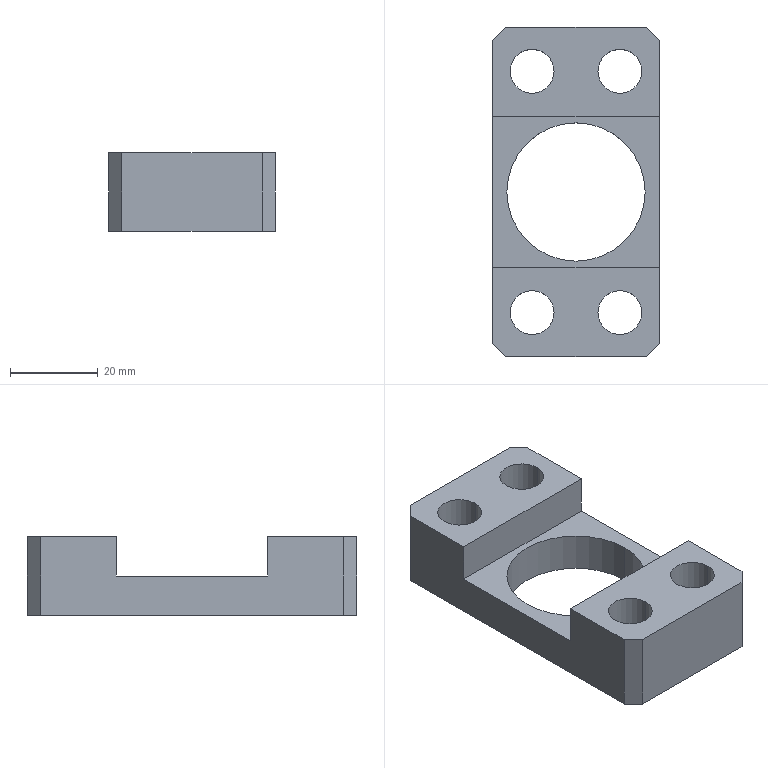Part | STEP file | Floating joint mounting plate | 1 solid | 36 faces | box 38 x 75 x 18 mm | volume 24096 mm3 | plane 18 | cylinder 18 | commonest cylinder face diameters 10 x8 14 x8 31.5 x2
STEP:
#1=CARTESIAN_POINT('',(34.75,37.5,9.));
#2=VERTEX_POINT('',#1);
#3=CARTESIAN_POINT('',(3.25,37.5,9.));
#4=VERTEX_POINT('',#3);
#5=CARTESIAN_POINT('',(19.,37.5,9.));
#6=DIRECTION('',(0.,0.,1.));
#7=DIRECTION('',(1.,0.,0.));
#8=AXIS2_PLACEMENT_3D('',#5,#6,#7);
#9=CIRCLE('',#8,15.75);
#10=EDGE_CURVE('',#2,#4,#9,.T.);
#11=ORIENTED_EDGE('',*,*,#10,.F.);
#12=CARTESIAN_POINT('',(19.,37.5,9.));
#13=DIRECTION('',(0.,0.,1.));
#14=DIRECTION('',(1.,0.,0.));
#15=AXIS2_PLACEMENT_3D('',#12,#13,#14);
#16=CIRCLE('',#15,15.75);
#17=EDGE_CURVE('',#4,#2,#16,.T.);
#18=ORIENTED_EDGE('',*,*,#17,.F.);
#19=EDGE_LOOP('',(#11,#18));
#20=FACE_BOUND('',#19,.T.);
#21=CARTESIAN_POINT('',(0.,20.25,9.));
#22=VERTEX_POINT('',#21);
#23=CARTESIAN_POINT('',(0.,54.75,9.));
#24=VERTEX_POINT('',#23);
#25=CARTESIAN_POINT('',(0.,20.25,9.));
#26=DIRECTION('',(0.,1.,0.));
#27=VECTOR('',#26,1000.);
#28=LINE('',#25,#27);
#29=EDGE_CURVE('',#22,#24,#28,.T.);
#30=ORIENTED_EDGE('',*,*,#29,.F.);
#31=CARTESIAN_POINT('',(38.,20.25,9.));
#32=VERTEX_POINT('',#31);
#33=CARTESIAN_POINT('',(38.,20.25,9.));
#34=DIRECTION('',(-1.,0.,0.));
#35=VECTOR('',#34,1000.);
#36=LINE('',#33,#35);
#37=EDGE_CURVE('',#32,#22,#36,.T.);
#38=ORIENTED_EDGE('',*,*,#37,.F.);
#39=CARTESIAN_POINT('',(38.,54.75,9.));
#40=VERTEX_POINT('',#39);
#41=CARTESIAN_POINT('',(38.,20.25,9.));
#42=DIRECTION('',(0.,1.,0.));
#43=VECTOR('',#42,1000.);
#44=LINE('',#41,#43);
#45=EDGE_CURVE('',#32,#40,#44,.T.);
#46=ORIENTED_EDGE('',*,*,#45,.T.);
#47=CARTESIAN_POINT('',(38.,54.75,9.));
#48=DIRECTION('',(-1.,0.,0.));
#49=VECTOR('',#48,1000.);
#50=LINE('',#47,#49);
#51=EDGE_CURVE('',#40,#24,#50,.T.);
#52=ORIENTED_EDGE('',*,*,#51,.T.);
#53=EDGE_LOOP('',(#30,#38,#46,#52));
#54=FACE_OUTER_BOUND('',#53,.T.);
#55=CARTESIAN_POINT('',(38.,20.25,9.));
#56=DIRECTION('',(0.,0.,1.));
#57=DIRECTION('',(1.,0.,0.));
#58=AXIS2_PLACEMENT_3D('',#55,#56,#57);
#59=PLANE('',#58);
#60=ADVANCED_FACE('',(#20,#54),#59,.T.);
#61=CARTESIAN_POINT('',(0.,54.75,18.));
#62=VERTEX_POINT('',#61);
#63=CARTESIAN_POINT('',(0.,54.75,9.));
#64=DIRECTION('',(0.,0.,1.));
#65=VECTOR('',#64,1000.);
#66=LINE('',#63,#65);
#67=EDGE_CURVE('',#24,#62,#66,.T.);
#68=ORIENTED_EDGE('',*,*,#67,.F.);
#69=ORIENTED_EDGE('',*,*,#51,.F.);
#70=CARTESIAN_POINT('',(38.,54.75,18.));
#71=VERTEX_POINT('',#70);
#72=CARTESIAN_POINT('',(38.,54.75,9.));
#73=DIRECTION('',(0.,0.,1.));
#74=VECTOR('',#73,1000.);
#75=LINE('',#72,#74);
#76=EDGE_CURVE('',#40,#71,#75,.T.);
#77=ORIENTED_EDGE('',*,*,#76,.T.);
#78=CARTESIAN_POINT('',(0.,54.75,18.));
#79=DIRECTION('',(1.,0.,0.));
#80=VECTOR('',#79,1000.);
#81=LINE('',#78,#80);
#82=EDGE_CURVE('',#62,#71,#81,.T.);
#83=ORIENTED_EDGE('',*,*,#82,.F.);
#84=EDGE_LOOP('',(#68,#69,#77,#83));
#85=FACE_OUTER_BOUND('',#84,.T.);
#86=CARTESIAN_POINT('',(38.,54.75,9.));
#87=DIRECTION('',(0.,-1.,0.));
#88=DIRECTION('',(0.,0.,-1.));
#89=AXIS2_PLACEMENT_3D('',#86,#87,#88);
#90=PLANE('',#89);
#91=ADVANCED_FACE('',(#85),#90,.T.);
#92=CARTESIAN_POINT('',(24.,65.,18.));
#93=VERTEX_POINT('',#92);
#94=CARTESIAN_POINT('',(34.,65.,18.));
#95=VERTEX_POINT('',#94);
#96=CARTESIAN_POINT('',(29.,65.,18.));
#97=DIRECTION('',(0.,0.,-1.));
#98=DIRECTION('',(-1.,0.,0.));
#99=AXIS2_PLACEMENT_3D('',#96,#97,#98);
#100=CIRCLE('',#99,5.);
#101=EDGE_CURVE('',#93,#95,#100,.T.);
#102=ORIENTED_EDGE('',*,*,#101,.T.);
#103=CARTESIAN_POINT('',(29.,65.,18.));
#104=DIRECTION('',(0.,0.,-1.));
#105=DIRECTION('',(-1.,0.,0.));
#106=AXIS2_PLACEMENT_3D('',#103,#104,#105);
#107=CIRCLE('',#106,5.);
#108=EDGE_CURVE('',#95,#93,#107,.T.);
#109=ORIENTED_EDGE('',*,*,#108,.T.);
#110=EDGE_LOOP('',(#102,#109));
#111=FACE_BOUND('',#110,.T.);
#112=CARTESIAN_POINT('',(4.,65.,18.));
#113=VERTEX_POINT('',#112);
#114=CARTESIAN_POINT('',(14.,65.,18.));
#115=VERTEX_POINT('',#114);
#116=CARTESIAN_POINT('',(9.,65.,18.));
#117=DIRECTION('',(0.,0.,-1.));
#118=DIRECTION('',(-1.,0.,0.));
#119=AXIS2_PLACEMENT_3D('',#116,#117,#118);
#120=CIRCLE('',#119,5.);
#121=EDGE_CURVE('',#113,#115,#120,.T.);
#122=ORIENTED_EDGE('',*,*,#121,.T.);
#123=CARTESIAN_POINT('',(9.,65.,18.));
#124=DIRECTION('',(0.,0.,-1.));
#125=DIRECTION('',(-1.,0.,0.));
#126=AXIS2_PLACEMENT_3D('',#123,#124,#125);
#127=CIRCLE('',#126,5.);
#128=EDGE_CURVE('',#115,#113,#127,.T.);
#129=ORIENTED_EDGE('',*,*,#128,.T.);
#130=EDGE_LOOP('',(#122,#129));
#131=FACE_BOUND('',#130,.T.);
#132=CARTESIAN_POINT('',(0.,72.,18.));
#133=VERTEX_POINT('',#132);
#134=CARTESIAN_POINT('',(0.,72.,18.));
#135=DIRECTION('',(0.,-1.,0.));
#136=VECTOR('',#135,1000.);
#137=LINE('',#134,#136);
#138=EDGE_CURVE('',#133,#62,#137,.T.);
#139=ORIENTED_EDGE('',*,*,#138,.T.);
#140=ORIENTED_EDGE('',*,*,#82,.T.);
#141=CARTESIAN_POINT('',(38.,72.,18.));
#142=VERTEX_POINT('',#141);
#143=CARTESIAN_POINT('',(38.,3.,18.));
#144=DIRECTION('',(0.,1.,0.));
#145=VECTOR('',#144,1000.);
#146=LINE('',#143,#145);
#147=EDGE_CURVE('',#71,#142,#146,.T.);
#148=ORIENTED_EDGE('',*,*,#147,.T.);
#149=CARTESIAN_POINT('',(35.,75.,18.));
#150=VERTEX_POINT('',#149);
#151=CARTESIAN_POINT('',(38.,72.,18.));
#152=DIRECTION('',(-0.7071,0.7071,0.));
#153=VECTOR('',#152,1000.);
#154=LINE('',#151,#153);
#155=EDGE_CURVE('',#142,#150,#154,.T.);
#156=ORIENTED_EDGE('',*,*,#155,.T.);
#157=CARTESIAN_POINT('',(3.,75.,18.));
#158=VERTEX_POINT('',#157);
#159=CARTESIAN_POINT('',(35.,75.,18.));
#160=DIRECTION('',(-1.,0.,0.));
#161=VECTOR('',#160,1000.);
#162=LINE('',#159,#161);
#163=EDGE_CURVE('',#150,#158,#162,.T.);
#164=ORIENTED_EDGE('',*,*,#163,.T.);
#165=CARTESIAN_POINT('',(3.,75.,18.));
#166=DIRECTION('',(-0.7071,-0.7071,0.));
#167=VECTOR('',#166,1000.);
#168=LINE('',#165,#167);
#169=EDGE_CURVE('',#158,#133,#168,.T.);
#170=ORIENTED_EDGE('',*,*,#169,.T.);
#171=EDGE_LOOP('',(#139,#140,#148,#156,#164,#170));
#172=FACE_OUTER_BOUND('',#171,.T.);
#173=CARTESIAN_POINT('',(0.,0.,18.));
#174=DIRECTION('',(0.,0.,1.));
#175=DIRECTION('',(1.,0.,0.));
#176=AXIS2_PLACEMENT_3D('',#173,#174,#175);
#177=PLANE('',#176);
#178=ADVANCED_FACE('',(#111,#131,#172),#177,.T.);
#179=CARTESIAN_POINT('',(3.,75.,0.));
#180=VERTEX_POINT('',#179);
#181=CARTESIAN_POINT('',(0.,72.,0.));
#182=VERTEX_POINT('',#181);
#183=CARTESIAN_POINT('',(3.,75.,0.));
#184=DIRECTION('',(-0.7071,-0.7071,0.));
#185=VECTOR('',#184,1000.);
#186=LINE('',#183,#185);
#187=EDGE_CURVE('',#180,#182,#186,.T.);
#188=ORIENTED_EDGE('',*,*,#187,.T.);
#189=CARTESIAN_POINT('',(0.,72.,18.));
#190=DIRECTION('',(0.,0.,-1.));
#191=VECTOR('',#190,1000.);
#192=LINE('',#189,#191);
#193=EDGE_CURVE('',#133,#182,#192,.T.);
#194=ORIENTED_EDGE('',*,*,#193,.F.);
#195=ORIENTED_EDGE('',*,*,#169,.F.);
#196=CARTESIAN_POINT('',(3.,75.,18.));
#197=DIRECTION('',(0.,0.,-1.));
#198=VECTOR('',#197,1000.);
#199=LINE('',#196,#198);
#200=EDGE_CURVE('',#158,#180,#199,.T.);
#201=ORIENTED_EDGE('',*,*,#200,.T.);
#202=EDGE_LOOP('',(#188,#194,#195,#201));
#203=FACE_OUTER_BOUND('',#202,.T.);
#204=CARTESIAN_POINT('',(3.,75.,18.));
#205=DIRECTION('',(0.7071,-0.7071,0.));
#206=DIRECTION('',(0.7071,0.7071,0.));
#207=AXIS2_PLACEMENT_3D('',#204,#205,#206);
#208=PLANE('',#207);
#209=ADVANCED_FACE('',(#203),#208,.F.);
#210=CARTESIAN_POINT('',(35.,75.,0.));
#211=VERTEX_POINT('',#210);
#212=CARTESIAN_POINT('',(35.,75.,0.));
#213=DIRECTION('',(-1.,0.,0.));
#214=VECTOR('',#213,1000.);
#215=LINE('',#212,#214);
#216=EDGE_CURVE('',#211,#180,#215,.T.);
#217=ORIENTED_EDGE('',*,*,#216,.T.);
#218=ORIENTED_EDGE('',*,*,#200,.F.);
#219=ORIENTED_EDGE('',*,*,#163,.F.);
#220=CARTESIAN_POINT('',(35.,75.,18.));
#221=DIRECTION('',(0.,0.,-1.));
#222=VECTOR('',#221,1000.);
#223=LINE('',#220,#222);
#224=EDGE_CURVE('',#150,#211,#223,.T.);
#225=ORIENTED_EDGE('',*,*,#224,.T.);
#226=EDGE_LOOP('',(#217,#218,#219,#225));
#227=FACE_OUTER_BOUND('',#226,.T.);
#228=CARTESIAN_POINT('',(35.,75.,18.));
#229=DIRECTION('',(0.,-1.,0.));
#230=DIRECTION('',(0.,0.,-1.));
#231=AXIS2_PLACEMENT_3D('',#228,#229,#230);
#232=PLANE('',#231);
#233=ADVANCED_FACE('',(#227),#232,.F.);
#234=CARTESIAN_POINT('',(38.,72.,0.));
#235=VERTEX_POINT('',#234);
#236=CARTESIAN_POINT('',(38.,72.,0.));
#237=DIRECTION('',(-0.7071,0.7071,0.));
#238=VECTOR('',#237,1000.);
#239=LINE('',#236,#238);
#240=EDGE_CURVE('',#235,#211,#239,.T.);
#241=ORIENTED_EDGE('',*,*,#240,.T.);
#242=ORIENTED_EDGE('',*,*,#224,.F.);
#243=ORIENTED_EDGE('',*,*,#155,.F.);
#244=CARTESIAN_POINT('',(38.,72.,18.));
#245=DIRECTION('',(0.,0.,-1.));
#246=VECTOR('',#245,1000.);
#247=LINE('',#244,#246);
#248=EDGE_CURVE('',#142,#235,#247,.T.);
#249=ORIENTED_EDGE('',*,*,#248,.T.);
#250=EDGE_LOOP('',(#241,#242,#243,#249));
#251=FACE_OUTER_BOUND('',#250,.T.);
#252=CARTESIAN_POINT('',(38.,72.,18.));
#253=DIRECTION('',(-0.7071,-0.7071,0.));
#254=DIRECTION('',(0.7071,-0.7071,0.));
#255=AXIS2_PLACEMENT_3D('',#252,#253,#254);
#256=PLANE('',#255);
#257=ADVANCED_FACE('',(#251),#256,.F.);
#258=ORIENTED_EDGE('',*,*,#76,.F.);
#259=ORIENTED_EDGE('',*,*,#45,.F.);
#260=CARTESIAN_POINT('',(38.,20.25,18.));
#261=VERTEX_POINT('',#260);
#262=CARTESIAN_POINT('',(38.,20.25,22.5));
#263=DIRECTION('',(0.,0.,-1.));
#264=VECTOR('',#263,1000.);
#265=LINE('',#262,#264);
#266=EDGE_CURVE('',#261,#32,#265,.T.);
#267=ORIENTED_EDGE('',*,*,#266,.F.);
#268=CARTESIAN_POINT('',(38.,3.,18.));
#269=VERTEX_POINT('',#268);
#270=CARTESIAN_POINT('',(38.,3.,18.));
#271=DIRECTION('',(0.,1.,0.));
#272=VECTOR('',#271,1000.);
#273=LINE('',#270,#272);
#274=EDGE_CURVE('',#269,#261,#273,.T.);
#275=ORIENTED_EDGE('',*,*,#274,.F.);
#276=CARTESIAN_POINT('',(38.,3.,0.));
#277=VERTEX_POINT('',#276);
#278=CARTESIAN_POINT('',(38.,3.,18.));
#279=DIRECTION('',(0.,0.,-1.));
#280=VECTOR('',#279,1000.);
#281=LINE('',#278,#280);
#282=EDGE_CURVE('',#269,#277,#281,.T.);
#283=ORIENTED_EDGE('',*,*,#282,.T.);
#284=CARTESIAN_POINT('',(38.,3.,0.));
#285=DIRECTION('',(0.,1.,0.));
#286=VECTOR('',#285,1000.);
#287=LINE('',#284,#286);
#288=EDGE_CURVE('',#277,#235,#287,.T.);
#289=ORIENTED_EDGE('',*,*,#288,.T.);
#290=ORIENTED_EDGE('',*,*,#248,.F.);
#291=ORIENTED_EDGE('',*,*,#147,.F.);
#292=EDGE_LOOP('',(#258,#259,#267,#275,#283,#289,#290,#291));
#293=FACE_OUTER_BOUND('',#292,.T.);
#294=CARTESIAN_POINT('',(38.,3.,18.));
#295=DIRECTION('',(-1.,0.,0.));
#296=DIRECTION('',(0.,0.,1.));
#297=AXIS2_PLACEMENT_3D('',#294,#295,#296);
#298=PLANE('',#297);
#299=ADVANCED_FACE('',(#293),#298,.F.);
#300=CARTESIAN_POINT('',(22.,65.,0.));
#301=VERTEX_POINT('',#300);
#302=CARTESIAN_POINT('',(36.,65.,0.));
#303=VERTEX_POINT('',#302);
#304=CARTESIAN_POINT('',(29.,65.,0.));
#305=DIRECTION('',(0.,0.,-1.));
#306=DIRECTION('',(-1.,0.,0.));
#307=AXIS2_PLACEMENT_3D('',#304,#305,#306);
#308=CIRCLE('',#307,7.);
#309=EDGE_CURVE('',#301,#303,#308,.T.);
#310=ORIENTED_EDGE('',*,*,#309,.F.);
#311=CARTESIAN_POINT('',(29.,65.,0.));
#312=DIRECTION('',(0.,0.,-1.));
#313=DIRECTION('',(-1.,0.,0.));
#314=AXIS2_PLACEMENT_3D('',#311,#312,#313);
#315=CIRCLE('',#314,7.);
#316=EDGE_CURVE('',#303,#301,#315,.T.);
#317=ORIENTED_EDGE('',*,*,#316,.F.);
#318=EDGE_LOOP('',(#310,#317));
#319=FACE_BOUND('',#318,.T.);
#320=CARTESIAN_POINT('',(2.,10.,0.));
#321=VERTEX_POINT('',#320);
#322=CARTESIAN_POINT('',(16.,10.,0.));
#323=VERTEX_POINT('',#322);
#324=CARTESIAN_POINT('',(9.,10.,0.));
#325=DIRECTION('',(0.,0.,-1.));
#326=DIRECTION('',(-1.,0.,0.));
#327=AXIS2_PLACEMENT_3D('',#324,#325,#326);
#328=CIRCLE('',#327,7.);
#329=EDGE_CURVE('',#321,#323,#328,.T.);
#330=ORIENTED_EDGE('',*,*,#329,.F.);
#331=CARTESIAN_POINT('',(9.,10.,0.));
#332=DIRECTION('',(0.,0.,-1.));
#333=DIRECTION('',(-1.,0.,0.));
#334=AXIS2_PLACEMENT_3D('',#331,#332,#333);
#335=CIRCLE('',#334,7.);
#336=EDGE_CURVE('',#323,#321,#335,.T.);
#337=ORIENTED_EDGE('',*,*,#336,.F.);
#338=EDGE_LOOP('',(#330,#337));
#339=FACE_BOUND('',#338,.T.);
#340=CARTESIAN_POINT('',(22.,10.,0.));
#341=VERTEX_POINT('',#340);
#342=CARTESIAN_POINT('',(36.,10.,0.));
#343=VERTEX_POINT('',#342);
#344=CARTESIAN_POINT('',(29.,10.,0.));
#345=DIRECTION('',(0.,0.,-1.));
#346=DIRECTION('',(-1.,0.,0.));
#347=AXIS2_PLACEMENT_3D('',#344,#345,#346);
#348=CIRCLE('',#347,7.);
#349=EDGE_CURVE('',#341,#343,#348,.T.);
#350=ORIENTED_EDGE('',*,*,#349,.F.);
#351=CARTESIAN_POINT('',(29.,10.,0.));
#352=DIRECTION('',(0.,0.,-1.));
#353=DIRECTION('',(-1.,0.,0.));
#354=AXIS2_PLACEMENT_3D('',#351,#352,#353);
#355=CIRCLE('',#354,7.);
#356=EDGE_CURVE('',#343,#341,#355,.T.);
#357=ORIENTED_EDGE('',*,*,#356,.F.);
#358=EDGE_LOOP('',(#350,#357));
#359=FACE_BOUND('',#358,.T.);
#360=CARTESIAN_POINT('',(2.,65.,0.));
#361=VERTEX_POINT('',#360);
#362=CARTESIAN_POINT('',(16.,65.,0.));
#363=VERTEX_POINT('',#362);
#364=CARTESIAN_POINT('',(9.,65.,0.));
#365=DIRECTION('',(0.,0.,-1.));
#366=DIRECTION('',(-1.,0.,0.));
#367=AXIS2_PLACEMENT_3D('',#364,#365,#366);
#368=CIRCLE('',#367,7.);
#369=EDGE_CURVE('',#361,#363,#368,.T.);
#370=ORIENTED_EDGE('',*,*,#369,.F.);
#371=CARTESIAN_POINT('',(9.,65.,0.));
#372=DIRECTION('',(0.,0.,-1.));
#373=DIRECTION('',(-1.,0.,0.));
#374=AXIS2_PLACEMENT_3D('',#371,#372,#373);
#375=CIRCLE('',#374,7.);
#376=EDGE_CURVE('',#363,#361,#375,.T.);
#377=ORIENTED_EDGE('',*,*,#376,.F.);
#378=EDGE_LOOP('',(#370,#377));
#379=FACE_BOUND('',#378,.T.);
#380=CARTESIAN_POINT('',(34.75,37.5,0.));
#381=VERTEX_POINT('',#380);
#382=CARTESIAN_POINT('',(3.25,37.5,0.));
#383=VERTEX_POINT('',#382);
#384=CARTESIAN_POINT('',(19.,37.5,0.));
#385=DIRECTION('',(0.,0.,1.));
#386=DIRECTION('',(1.,0.,0.));
#387=AXIS2_PLACEMENT_3D('',#384,#385,#386);
#388=CIRCLE('',#387,15.75);
#389=EDGE_CURVE('',#381,#383,#388,.T.);
#390=ORIENTED_EDGE('',*,*,#389,.T.);
#391=CARTESIAN_POINT('',(19.,37.5,0.));
#392=DIRECTION('',(0.,0.,1.));
#393=DIRECTION('',(1.,0.,0.));
#394=AXIS2_PLACEMENT_3D('',#391,#392,#393);
#395=CIRCLE('',#394,15.75);
#396=EDGE_CURVE('',#383,#381,#395,.T.);
#397=ORIENTED_EDGE('',*,*,#396,.T.);
#398=EDGE_LOOP('',(#390,#397));
#399=FACE_BOUND('',#398,.T.);
#400=CARTESIAN_POINT('',(0.,3.,0.));
#401=VERTEX_POINT('',#400);
#402=CARTESIAN_POINT('',(0.,72.,0.));
#403=DIRECTION('',(0.,-1.,0.));
#404=VECTOR('',#403,1000.);
#405=LINE('',#402,#404);
#406=EDGE_CURVE('',#182,#401,#405,.T.);
#407=ORIENTED_EDGE('',*,*,#406,.F.);
#408=ORIENTED_EDGE('',*,*,#187,.F.);
#409=ORIENTED_EDGE('',*,*,#216,.F.);
#410=ORIENTED_EDGE('',*,*,#240,.F.);
#411=ORIENTED_EDGE('',*,*,#288,.F.);
#412=CARTESIAN_POINT('',(35.,0.,0.));
#413=VERTEX_POINT('',#412);
#414=CARTESIAN_POINT('',(35.,0.,0.));
#415=DIRECTION('',(0.7071,0.7071,0.));
#416=VECTOR('',#415,1000.);
#417=LINE('',#414,#416);
#418=EDGE_CURVE('',#413,#277,#417,.T.);
#419=ORIENTED_EDGE('',*,*,#418,.F.);
#420=CARTESIAN_POINT('',(3.,0.,0.));
#421=VERTEX_POINT('',#420);
#422=CARTESIAN_POINT('',(3.,0.,0.));
#423=DIRECTION('',(1.,0.,0.));
#424=VECTOR('',#423,1000.);
#425=LINE('',#422,#424);
#426=EDGE_CURVE('',#421,#413,#425,.T.);
#427=ORIENTED_EDGE('',*,*,#426,.F.);
#428=CARTESIAN_POINT('',(0.,3.,0.));
#429=DIRECTION('',(0.7071,-0.7071,0.));
#430=VECTOR('',#429,1000.);
#431=LINE('',#428,#430);
#432=EDGE_CURVE('',#401,#421,#431,.T.);
#433=ORIENTED_EDGE('',*,*,#432,.F.);
#434=EDGE_LOOP('',(#407,#408,#409,#410,#411,#419,#427,#433));
#435=FACE_OUTER_BOUND('',#434,.T.);
#436=CARTESIAN_POINT('',(0.,0.,0.));
#437=DIRECTION('',(0.,0.,1.));
#438=DIRECTION('',(1.,0.,0.));
#439=AXIS2_PLACEMENT_3D('',#436,#437,#438);
#440=PLANE('',#439);
#441=ADVANCED_FACE('',(#319,#339,#359,#379,#399,#435),#440,.F.);
#442=ORIENTED_EDGE('',*,*,#432,.T.);
#443=CARTESIAN_POINT('',(3.,0.,18.));
#444=VERTEX_POINT('',#443);
#445=CARTESIAN_POINT('',(3.,0.,18.));
#446=DIRECTION('',(0.,0.,-1.));
#447=VECTOR('',#446,1000.);
#448=LINE('',#445,#447);
#449=EDGE_CURVE('',#444,#421,#448,.T.);
#450=ORIENTED_EDGE('',*,*,#449,.F.);
#451=CARTESIAN_POINT('',(0.,3.,18.));
#452=VERTEX_POINT('',#451);
#453=CARTESIAN_POINT('',(0.,3.,18.));
#454=DIRECTION('',(0.7071,-0.7071,0.));
#455=VECTOR('',#454,1000.);
#456=LINE('',#453,#455);
#457=EDGE_CURVE('',#452,#444,#456,.T.);
#458=ORIENTED_EDGE('',*,*,#457,.F.);
#459=CARTESIAN_POINT('',(0.,3.,18.));
#460=DIRECTION('',(0.,0.,-1.));
#461=VECTOR('',#460,1000.);
#462=LINE('',#459,#461);
#463=EDGE_CURVE('',#452,#401,#462,.T.);
#464=ORIENTED_EDGE('',*,*,#463,.T.);
#465=EDGE_LOOP('',(#442,#450,#458,#464));
#466=FACE_OUTER_BOUND('',#465,.T.);
#467=CARTESIAN_POINT('',(0.,3.,18.));
#468=DIRECTION('',(0.7071,0.7071,0.));
#469=DIRECTION('',(-0.7071,0.7071,0.));
#470=AXIS2_PLACEMENT_3D('',#467,#468,#469);
#471=PLANE('',#470);
#472=ADVANCED_FACE('',(#466),#471,.F.);
#473=ORIENTED_EDGE('',*,*,#67,.T.);
#474=ORIENTED_EDGE('',*,*,#138,.F.);
#475=ORIENTED_EDGE('',*,*,#193,.T.);
#476=ORIENTED_EDGE('',*,*,#406,.T.);
#477=ORIENTED_EDGE('',*,*,#463,.F.);
#478=CARTESIAN_POINT('',(0.,20.25,18.));
#479=VERTEX_POINT('',#478);
#480=CARTESIAN_POINT('',(0.,72.,18.));
#481=DIRECTION('',(0.,-1.,0.));
#482=VECTOR('',#481,1000.);
#483=LINE('',#480,#482);
#484=EDGE_CURVE('',#479,#452,#483,.T.);
#485=ORIENTED_EDGE('',*,*,#484,.F.);
#486=CARTESIAN_POINT('',(0.,20.25,22.5));
#487=DIRECTION('',(0.,0.,-1.));
#488=VECTOR('',#487,1000.);
#489=LINE('',#486,#488);
#490=EDGE_CURVE('',#479,#22,#489,.T.);
#491=ORIENTED_EDGE('',*,*,#490,.T.);
#492=ORIENTED_EDGE('',*,*,#29,.T.);
#493=EDGE_LOOP('',(#473,#474,#475,#476,#477,#485,#491,#492));
#494=FACE_OUTER_BOUND('',#493,.T.);
#495=CARTESIAN_POINT('',(0.,72.,18.));
#496=DIRECTION('',(1.,0.,0.));
#497=DIRECTION('',(0.,0.,-1.));
#498=AXIS2_PLACEMENT_3D('',#495,#496,#497);
#499=PLANE('',#498);
#500=ADVANCED_FACE('',(#494),#499,.F.);
#501=ORIENTED_EDGE('',*,*,#266,.T.);
#502=ORIENTED_EDGE('',*,*,#37,.T.);
#503=ORIENTED_EDGE('',*,*,#490,.F.);
#504=CARTESIAN_POINT('',(0.,20.25,18.));
#505=DIRECTION('',(-1.,0.,0.));
#506=VECTOR('',#505,1000.);
#507=LINE('',#504,#506);
#508=EDGE_CURVE('',#261,#479,#507,.T.);
#509=ORIENTED_EDGE('',*,*,#508,.F.);
#510=EDGE_LOOP('',(#501,#502,#503,#509));
#511=FACE_OUTER_BOUND('',#510,.T.);
#512=CARTESIAN_POINT('',(38.,20.25,22.5));
#513=DIRECTION('',(0.,1.,0.));
#514=DIRECTION('',(0.,0.,1.));
#515=AXIS2_PLACEMENT_3D('',#512,#513,#514);
#516=PLANE('',#515);
#517=ADVANCED_FACE('',(#511),#516,.T.);
#518=CARTESIAN_POINT('',(4.,10.,18.));
#519=VERTEX_POINT('',#518);
#520=CARTESIAN_POINT('',(14.,10.,18.));
#521=VERTEX_POINT('',#520);
#522=CARTESIAN_POINT('',(9.,10.,18.));
#523=DIRECTION('',(0.,0.,-1.));
#524=DIRECTION('',(-1.,0.,0.));
#525=AXIS2_PLACEMENT_3D('',#522,#523,#524);
#526=CIRCLE('',#525,5.);
#527=EDGE_CURVE('',#519,#521,#526,.T.);
#528=ORIENTED_EDGE('',*,*,#527,.T.);
#529=CARTESIAN_POINT('',(9.,10.,18.));
#530=DIRECTION('',(0.,0.,-1.));
#531=DIRECTION('',(-1.,0.,0.));
#532=AXIS2_PLACEMENT_3D('',#529,#530,#531);
#533=CIRCLE('',#532,5.);
#534=EDGE_CURVE('',#521,#519,#533,.T.);
#535=ORIENTED_EDGE('',*,*,#534,.T.);
#536=EDGE_LOOP('',(#528,#535));
#537=FACE_BOUND('',#536,.T.);
#538=CARTESIAN_POINT('',(24.,10.,18.));
#539=VERTEX_POINT('',#538);
#540=CARTESIAN_POINT('',(34.,10.,18.));
#541=VERTEX_POINT('',#540);
#542=CARTESIAN_POINT('',(29.,10.,18.));
#543=DIRECTION('',(0.,0.,-1.));
#544=DIRECTION('',(-1.,0.,0.));
#545=AXIS2_PLACEMENT_3D('',#542,#543,#544);
#546=CIRCLE('',#545,5.);
#547=EDGE_CURVE('',#539,#541,#546,.T.);
#548=ORIENTED_EDGE('',*,*,#547,.T.);
#549=CARTESIAN_POINT('',(29.,10.,18.));
#550=DIRECTION('',(0.,0.,-1.));
#551=DIRECTION('',(-1.,0.,0.));
#552=AXIS2_PLACEMENT_3D('',#549,#550,#551);
#553=CIRCLE('',#552,5.);
#554=EDGE_CURVE('',#541,#539,#553,.T.);
#555=ORIENTED_EDGE('',*,*,#554,.T.);
#556=EDGE_LOOP('',(#548,#555));
#557=FACE_BOUND('',#556,.T.);
#558=ORIENTED_EDGE('',*,*,#274,.T.);
#559=ORIENTED_EDGE('',*,*,#508,.T.);
#560=ORIENTED_EDGE('',*,*,#484,.T.);
#561=ORIENTED_EDGE('',*,*,#457,.T.);
#562=CARTESIAN_POINT('',(35.,0.,18.));
#563=VERTEX_POINT('',#562);
#564=CARTESIAN_POINT('',(3.,0.,18.));
#565=DIRECTION('',(1.,0.,0.));
#566=VECTOR('',#565,1000.);
#567=LINE('',#564,#566);
#568=EDGE_CURVE('',#444,#563,#567,.T.);
#569=ORIENTED_EDGE('',*,*,#568,.T.);
#570=CARTESIAN_POINT('',(35.,0.,18.));
#571=DIRECTION('',(0.7071,0.7071,0.));
#572=VECTOR('',#571,1000.);
#573=LINE('',#570,#572);
#574=EDGE_CURVE('',#563,#269,#573,.T.);
#575=ORIENTED_EDGE('',*,*,#574,.T.);
#576=EDGE_LOOP('',(#558,#559,#560,#561,#569,#575));
#577=FACE_OUTER_BOUND('',#576,.T.);
#578=CARTESIAN_POINT('',(0.,0.,18.));
#579=DIRECTION('',(0.,0.,1.));
#580=DIRECTION('',(1.,0.,0.));
#581=AXIS2_PLACEMENT_3D('',#578,#579,#580);
#582=PLANE('',#581);
#583=ADVANCED_FACE('',(#537,#557,#577),#582,.T.);
#584=ORIENTED_EDGE('',*,*,#418,.T.);
#585=ORIENTED_EDGE('',*,*,#282,.F.);
#586=ORIENTED_EDGE('',*,*,#574,.F.);
#587=CARTESIAN_POINT('',(35.,0.,18.));
#588=DIRECTION('',(0.,0.,-1.));
#589=VECTOR('',#588,1000.);
#590=LINE('',#587,#589);
#591=EDGE_CURVE('',#563,#413,#590,.T.);
#592=ORIENTED_EDGE('',*,*,#591,.T.);
#593=EDGE_LOOP('',(#584,#585,#586,#592));
#594=FACE_OUTER_BOUND('',#593,.T.);
#595=CARTESIAN_POINT('',(35.,0.,18.));
#596=DIRECTION('',(-0.7071,0.7071,0.));
#597=DIRECTION('',(-0.7071,-0.7071,0.));
#598=AXIS2_PLACEMENT_3D('',#595,#596,#597);
#599=PLANE('',#598);
#600=ADVANCED_FACE('',(#594),#599,.F.);
#601=ORIENTED_EDGE('',*,*,#426,.T.);
#602=ORIENTED_EDGE('',*,*,#591,.F.);
#603=ORIENTED_EDGE('',*,*,#568,.F.);
#604=ORIENTED_EDGE('',*,*,#449,.T.);
#605=EDGE_LOOP('',(#601,#602,#603,#604));
#606=FACE_OUTER_BOUND('',#605,.T.);
#607=CARTESIAN_POINT('',(3.,0.,18.));
#608=DIRECTION('',(0.,1.,0.));
#609=DIRECTION('',(0.,0.,1.));
#610=AXIS2_PLACEMENT_3D('',#607,#608,#609);
#611=PLANE('',#610);
#612=ADVANCED_FACE('',(#606),#611,.F.);
#613=ORIENTED_EDGE('',*,*,#554,.F.);
#614=CARTESIAN_POINT('',(34.,10.,8.));
#615=VERTEX_POINT('',#614);
#616=CARTESIAN_POINT('',(34.,10.,8.));
#617=DIRECTION('',(0.,0.,1.));
#618=VECTOR('',#617,1000.);
#619=LINE('',#616,#618);
#620=EDGE_CURVE('',#615,#541,#619,.T.);
#621=ORIENTED_EDGE('',*,*,#620,.F.);
#622=CARTESIAN_POINT('',(24.,10.,8.));
#623=VERTEX_POINT('',#622);
#624=CARTESIAN_POINT('',(29.,10.,8.));
#625=DIRECTION('',(0.,0.,-1.));
#626=DIRECTION('',(-1.,0.,0.));
#627=AXIS2_PLACEMENT_3D('',#624,#625,#626);
#628=CIRCLE('',#627,5.);
#629=EDGE_CURVE('',#615,#623,#628,.T.);
#630=ORIENTED_EDGE('',*,*,#629,.T.);
#631=CARTESIAN_POINT('',(24.,10.,8.));
#632=DIRECTION('',(0.,0.,1.));
#633=VECTOR('',#632,1000.);
#634=LINE('',#631,#633);
#635=EDGE_CURVE('',#623,#539,#634,.T.);
#636=ORIENTED_EDGE('',*,*,#635,.T.);
#637=EDGE_LOOP('',(#613,#621,#630,#636));
#638=FACE_OUTER_BOUND('',#637,.T.);
#639=CARTESIAN_POINT('',(29.,10.,0.));
#640=DIRECTION('',(0.,0.,1.));
#641=DIRECTION('',(0.,1.,0.));
#642=AXIS2_PLACEMENT_3D('',#639,#640,#641);
#643=CYLINDRICAL_SURFACE('',#642,5.);
#644=ADVANCED_FACE('',(#638),#643,.F.);
#645=CARTESIAN_POINT('',(29.,10.,8.));
#646=DIRECTION('',(0.,0.,-1.));
#647=DIRECTION('',(-1.,0.,0.));
#648=AXIS2_PLACEMENT_3D('',#645,#646,#647);
#649=CIRCLE('',#648,5.);
#650=EDGE_CURVE('',#623,#615,#649,.T.);
#651=ORIENTED_EDGE('',*,*,#650,.T.);
#652=ORIENTED_EDGE('',*,*,#620,.T.);
#653=ORIENTED_EDGE('',*,*,#547,.F.);
#654=ORIENTED_EDGE('',*,*,#635,.F.);
#655=EDGE_LOOP('',(#651,#652,#653,#654));
#656=FACE_OUTER_BOUND('',#655,.T.);
#657=CARTESIAN_POINT('',(29.,10.,0.));
#658=DIRECTION('',(0.,0.,1.));
#659=DIRECTION('',(0.,-1.,0.));
#660=AXIS2_PLACEMENT_3D('',#657,#658,#659);
#661=CYLINDRICAL_SURFACE('',#660,5.);
#662=ADVANCED_FACE('',(#656),#661,.F.);
#663=CARTESIAN_POINT('',(22.,10.,8.));
#664=VERTEX_POINT('',#663);
#665=CARTESIAN_POINT('',(36.,10.,8.));
#666=VERTEX_POINT('',#665);
#667=CARTESIAN_POINT('',(29.,10.,8.));
#668=DIRECTION('',(0.,0.,-1.));
#669=DIRECTION('',(-1.,0.,0.));
#670=AXIS2_PLACEMENT_3D('',#667,#668,#669);
#671=CIRCLE('',#670,7.);
#672=EDGE_CURVE('',#664,#666,#671,.T.);
#673=ORIENTED_EDGE('',*,*,#672,.T.);
#674=CARTESIAN_POINT('',(29.,10.,8.));
#675=DIRECTION('',(0.,0.,-1.));
#676=DIRECTION('',(-1.,0.,0.));
#677=AXIS2_PLACEMENT_3D('',#674,#675,#676);
#678=CIRCLE('',#677,7.);
#679=EDGE_CURVE('',#666,#664,#678,.T.);
#680=ORIENTED_EDGE('',*,*,#679,.T.);
#681=EDGE_LOOP('',(#673,#680));
#682=FACE_OUTER_BOUND('',#681,.T.);
#683=ORIENTED_EDGE('',*,*,#650,.F.);
#684=ORIENTED_EDGE('',*,*,#629,.F.);
#685=EDGE_LOOP('',(#683,#684));
#686=FACE_BOUND('',#685,.T.);
#687=CARTESIAN_POINT('',(29.,15.,8.));
#688=DIRECTION('',(0.,0.,-1.));
#689=DIRECTION('',(-1.,0.,0.));
#690=AXIS2_PLACEMENT_3D('',#687,#688,#689);
#691=PLANE('',#690);
#692=ADVANCED_FACE('',(#682,#686),#691,.T.);
#693=ORIENTED_EDGE('',*,*,#679,.F.);
#694=CARTESIAN_POINT('',(36.,10.,0.));
#695=DIRECTION('',(0.,0.,1.));
#696=VECTOR('',#695,1000.);
#697=LINE('',#694,#696);
#698=EDGE_CURVE('',#343,#666,#697,.T.);
#699=ORIENTED_EDGE('',*,*,#698,.F.);
#700=ORIENTED_EDGE('',*,*,#356,.T.);
#701=CARTESIAN_POINT('',(22.,10.,0.));
#702=DIRECTION('',(0.,0.,1.));
#703=VECTOR('',#702,1000.);
#704=LINE('',#701,#703);
#705=EDGE_CURVE('',#341,#664,#704,.T.);
#706=ORIENTED_EDGE('',*,*,#705,.T.);
#707=EDGE_LOOP('',(#693,#699,#700,#706));
#708=FACE_OUTER_BOUND('',#707,.T.);
#709=CARTESIAN_POINT('',(29.,10.,0.));
#710=DIRECTION('',(0.,0.,1.));
#711=DIRECTION('',(0.,1.,0.));
#712=AXIS2_PLACEMENT_3D('',#709,#710,#711);
#713=CYLINDRICAL_SURFACE('',#712,7.);
#714=ADVANCED_FACE('',(#708),#713,.F.);
#715=ORIENTED_EDGE('',*,*,#349,.T.);
#716=ORIENTED_EDGE('',*,*,#698,.T.);
#717=ORIENTED_EDGE('',*,*,#672,.F.);
#718=ORIENTED_EDGE('',*,*,#705,.F.);
#719=EDGE_LOOP('',(#715,#716,#717,#718));
#720=FACE_OUTER_BOUND('',#719,.T.);
#721=CARTESIAN_POINT('',(29.,10.,0.));
#722=DIRECTION('',(0.,0.,1.));
#723=DIRECTION('',(0.,-1.,0.));
#724=AXIS2_PLACEMENT_3D('',#721,#722,#723);
#725=CYLINDRICAL_SURFACE('',#724,7.);
#726=ADVANCED_FACE('',(#720),#725,.F.);
#727=ORIENTED_EDGE('',*,*,#534,.F.);
#728=CARTESIAN_POINT('',(14.,10.,8.));
#729=VERTEX_POINT('',#728);
#730=CARTESIAN_POINT('',(14.,10.,8.));
#731=DIRECTION('',(0.,0.,1.));
#732=VECTOR('',#731,1000.);
#733=LINE('',#730,#732);
#734=EDGE_CURVE('',#729,#521,#733,.T.);
#735=ORIENTED_EDGE('',*,*,#734,.F.);
#736=CARTESIAN_POINT('',(4.,10.,8.));
#737=VERTEX_POINT('',#736);
#738=CARTESIAN_POINT('',(9.,10.,8.));
#739=DIRECTION('',(0.,0.,-1.));
#740=DIRECTION('',(-1.,0.,0.));
#741=AXIS2_PLACEMENT_3D('',#738,#739,#740);
#742=CIRCLE('',#741,5.);
#743=EDGE_CURVE('',#729,#737,#742,.T.);
#744=ORIENTED_EDGE('',*,*,#743,.T.);
#745=CARTESIAN_POINT('',(4.,10.,8.));
#746=DIRECTION('',(0.,0.,1.));
#747=VECTOR('',#746,1000.);
#748=LINE('',#745,#747);
#749=EDGE_CURVE('',#737,#519,#748,.T.);
#750=ORIENTED_EDGE('',*,*,#749,.T.);
#751=EDGE_LOOP('',(#727,#735,#744,#750));
#752=FACE_OUTER_BOUND('',#751,.T.);
#753=CARTESIAN_POINT('',(9.,10.,0.));
#754=DIRECTION('',(0.,0.,1.));
#755=DIRECTION('',(0.,1.,0.));
#756=AXIS2_PLACEMENT_3D('',#753,#754,#755);
#757=CYLINDRICAL_SURFACE('',#756,5.);
#758=ADVANCED_FACE('',(#752),#757,.F.);
#759=CARTESIAN_POINT('',(9.,10.,8.));
#760=DIRECTION('',(0.,0.,-1.));
#761=DIRECTION('',(-1.,0.,0.));
#762=AXIS2_PLACEMENT_3D('',#759,#760,#761);
#763=CIRCLE('',#762,5.);
#764=EDGE_CURVE('',#737,#729,#763,.T.);
#765=ORIENTED_EDGE('',*,*,#764,.T.);
#766=ORIENTED_EDGE('',*,*,#734,.T.);
#767=ORIENTED_EDGE('',*,*,#527,.F.);
#768=ORIENTED_EDGE('',*,*,#749,.F.);
#769=EDGE_LOOP('',(#765,#766,#767,#768));
#770=FACE_OUTER_BOUND('',#769,.T.);
#771=CARTESIAN_POINT('',(9.,10.,0.));
#772=DIRECTION('',(0.,0.,1.));
#773=DIRECTION('',(0.,-1.,0.));
#774=AXIS2_PLACEMENT_3D('',#771,#772,#773);
#775=CYLINDRICAL_SURFACE('',#774,5.);
#776=ADVANCED_FACE('',(#770),#775,.F.);
#777=CARTESIAN_POINT('',(2.,10.,8.));
#778=VERTEX_POINT('',#777);
#779=CARTESIAN_POINT('',(16.,10.,8.));
#780=VERTEX_POINT('',#779);
#781=CARTESIAN_POINT('',(9.,10.,8.));
#782=DIRECTION('',(0.,0.,-1.));
#783=DIRECTION('',(-1.,0.,0.));
#784=AXIS2_PLACEMENT_3D('',#781,#782,#783);
#785=CIRCLE('',#784,7.);
#786=EDGE_CURVE('',#778,#780,#785,.T.);
#787=ORIENTED_EDGE('',*,*,#786,.T.);
#788=CARTESIAN_POINT('',(9.,10.,8.));
#789=DIRECTION('',(0.,0.,-1.));
#790=DIRECTION('',(-1.,0.,0.));
#791=AXIS2_PLACEMENT_3D('',#788,#789,#790);
#792=CIRCLE('',#791,7.);
#793=EDGE_CURVE('',#780,#778,#792,.T.);
#794=ORIENTED_EDGE('',*,*,#793,.T.);
#795=EDGE_LOOP('',(#787,#794));
#796=FACE_OUTER_BOUND('',#795,.T.);
#797=ORIENTED_EDGE('',*,*,#764,.F.);
#798=ORIENTED_EDGE('',*,*,#743,.F.);
#799=EDGE_LOOP('',(#797,#798));
#800=FACE_BOUND('',#799,.T.);
#801=CARTESIAN_POINT('',(9.,15.,8.));
#802=DIRECTION('',(0.,0.,-1.));
#803=DIRECTION('',(-1.,0.,0.));
#804=AXIS2_PLACEMENT_3D('',#801,#802,#803);
#805=PLANE('',#804);
#806=ADVANCED_FACE('',(#796,#800),#805,.T.);
#807=ORIENTED_EDGE('',*,*,#793,.F.);
#808=CARTESIAN_POINT('',(16.,10.,0.));
#809=DIRECTION('',(0.,0.,1.));
#810=VECTOR('',#809,1000.);
#811=LINE('',#808,#810);
#812=EDGE_CURVE('',#323,#780,#811,.T.);
#813=ORIENTED_EDGE('',*,*,#812,.F.);
#814=ORIENTED_EDGE('',*,*,#336,.T.);
#815=CARTESIAN_POINT('',(2.,10.,0.));
#816=DIRECTION('',(0.,0.,1.));
#817=VECTOR('',#816,1000.);
#818=LINE('',#815,#817);
#819=EDGE_CURVE('',#321,#778,#818,.T.);
#820=ORIENTED_EDGE('',*,*,#819,.T.);
#821=EDGE_LOOP('',(#807,#813,#814,#820));
#822=FACE_OUTER_BOUND('',#821,.T.);
#823=CARTESIAN_POINT('',(9.,10.,0.));
#824=DIRECTION('',(0.,0.,1.));
#825=DIRECTION('',(0.,1.,0.));
#826=AXIS2_PLACEMENT_3D('',#823,#824,#825);
#827=CYLINDRICAL_SURFACE('',#826,7.);
#828=ADVANCED_FACE('',(#822),#827,.F.);
#829=ORIENTED_EDGE('',*,*,#329,.T.);
#830=ORIENTED_EDGE('',*,*,#812,.T.);
#831=ORIENTED_EDGE('',*,*,#786,.F.);
#832=ORIENTED_EDGE('',*,*,#819,.F.);
#833=EDGE_LOOP('',(#829,#830,#831,#832));
#834=FACE_OUTER_BOUND('',#833,.T.);
#835=CARTESIAN_POINT('',(9.,10.,0.));
#836=DIRECTION('',(0.,0.,1.));
#837=DIRECTION('',(0.,-1.,0.));
#838=AXIS2_PLACEMENT_3D('',#835,#836,#837);
#839=CYLINDRICAL_SURFACE('',#838,7.);
#840=ADVANCED_FACE('',(#834),#839,.F.);
#841=ORIENTED_EDGE('',*,*,#396,.F.);
#842=CARTESIAN_POINT('',(3.25,37.5,0.));
#843=DIRECTION('',(0.,0.,1.));
#844=VECTOR('',#843,1000.);
#845=LINE('',#842,#844);
#846=EDGE_CURVE('',#383,#4,#845,.T.);
#847=ORIENTED_EDGE('',*,*,#846,.T.);
#848=ORIENTED_EDGE('',*,*,#17,.T.);
#849=CARTESIAN_POINT('',(34.75,37.5,0.));
#850=DIRECTION('',(0.,0.,1.));
#851=VECTOR('',#850,1000.);
#852=LINE('',#849,#851);
#853=EDGE_CURVE('',#381,#2,#852,.T.);
#854=ORIENTED_EDGE('',*,*,#853,.F.);
#855=EDGE_LOOP('',(#841,#847,#848,#854));
#856=FACE_OUTER_BOUND('',#855,.T.);
#857=CARTESIAN_POINT('',(19.,37.5,18.));
#858=DIRECTION('',(0.,0.,1.));
#859=DIRECTION('',(0.,1.,0.));
#860=AXIS2_PLACEMENT_3D('',#857,#858,#859);
#861=CYLINDRICAL_SURFACE('',#860,15.75);
#862=ADVANCED_FACE('',(#856),#861,.F.);
#863=ORIENTED_EDGE('',*,*,#10,.T.);
#864=ORIENTED_EDGE('',*,*,#846,.F.);
#865=ORIENTED_EDGE('',*,*,#389,.F.);
#866=ORIENTED_EDGE('',*,*,#853,.T.);
#867=EDGE_LOOP('',(#863,#864,#865,#866));
#868=FACE_OUTER_BOUND('',#867,.T.);
#869=CARTESIAN_POINT('',(19.,37.5,18.));
#870=DIRECTION('',(0.,0.,1.));
#871=DIRECTION('',(0.,-1.,0.));
#872=AXIS2_PLACEMENT_3D('',#869,#870,#871);
#873=CYLINDRICAL_SURFACE('',#872,15.75);
#874=ADVANCED_FACE('',(#868),#873,.F.);
#875=CARTESIAN_POINT('',(16.,65.,8.));
#876=VERTEX_POINT('',#875);
#877=CARTESIAN_POINT('',(2.,65.,8.));
#878=VERTEX_POINT('',#877);
#879=CARTESIAN_POINT('',(9.,65.,8.));
#880=DIRECTION('',(0.,0.,-1.));
#881=DIRECTION('',(-1.,0.,0.));
#882=AXIS2_PLACEMENT_3D('',#879,#880,#881);
#883=CIRCLE('',#882,7.);
#884=EDGE_CURVE('',#876,#878,#883,.T.);
#885=ORIENTED_EDGE('',*,*,#884,.F.);
#886=CARTESIAN_POINT('',(16.,65.,0.));
#887=DIRECTION('',(0.,0.,1.));
#888=VECTOR('',#887,1000.);
#889=LINE('',#886,#888);
#890=EDGE_CURVE('',#363,#876,#889,.T.);
#891=ORIENTED_EDGE('',*,*,#890,.F.);
#892=ORIENTED_EDGE('',*,*,#376,.T.);
#893=CARTESIAN_POINT('',(2.,65.,0.));
#894=DIRECTION('',(0.,0.,1.));
#895=VECTOR('',#894,1000.);
#896=LINE('',#893,#895);
#897=EDGE_CURVE('',#361,#878,#896,.T.);
#898=ORIENTED_EDGE('',*,*,#897,.T.);
#899=EDGE_LOOP('',(#885,#891,#892,#898));
#900=FACE_OUTER_BOUND('',#899,.T.);
#901=CARTESIAN_POINT('',(9.,65.,0.));
#902=DIRECTION('',(0.,0.,1.));
#903=DIRECTION('',(0.,1.,0.));
#904=AXIS2_PLACEMENT_3D('',#901,#902,#903);
#905=CYLINDRICAL_SURFACE('',#904,7.);
#906=ADVANCED_FACE('',(#900),#905,.F.);
#907=ORIENTED_EDGE('',*,*,#369,.T.);
#908=ORIENTED_EDGE('',*,*,#890,.T.);
#909=CARTESIAN_POINT('',(9.,65.,8.));
#910=DIRECTION('',(0.,0.,-1.));
#911=DIRECTION('',(-1.,0.,0.));
#912=AXIS2_PLACEMENT_3D('',#909,#910,#911);
#913=CIRCLE('',#912,7.);
#914=EDGE_CURVE('',#878,#876,#913,.T.);
#915=ORIENTED_EDGE('',*,*,#914,.F.);
#916=ORIENTED_EDGE('',*,*,#897,.F.);
#917=EDGE_LOOP('',(#907,#908,#915,#916));
#918=FACE_OUTER_BOUND('',#917,.T.);
#919=CARTESIAN_POINT('',(9.,65.,0.));
#920=DIRECTION('',(0.,0.,1.));
#921=DIRECTION('',(0.,-1.,0.));
#922=AXIS2_PLACEMENT_3D('',#919,#920,#921);
#923=CYLINDRICAL_SURFACE('',#922,7.);
#924=ADVANCED_FACE('',(#918),#923,.F.);
#925=ORIENTED_EDGE('',*,*,#914,.T.);
#926=ORIENTED_EDGE('',*,*,#884,.T.);
#927=EDGE_LOOP('',(#925,#926));
#928=FACE_OUTER_BOUND('',#927,.T.);
#929=CARTESIAN_POINT('',(4.,65.,8.));
#930=VERTEX_POINT('',#929);
#931=CARTESIAN_POINT('',(14.,65.,8.));
#932=VERTEX_POINT('',#931);
#933=CARTESIAN_POINT('',(9.,65.,8.));
#934=DIRECTION('',(0.,0.,-1.));
#935=DIRECTION('',(-1.,0.,0.));
#936=AXIS2_PLACEMENT_3D('',#933,#934,#935);
#937=CIRCLE('',#936,5.);
#938=EDGE_CURVE('',#930,#932,#937,.T.);
#939=ORIENTED_EDGE('',*,*,#938,.F.);
#940=CARTESIAN_POINT('',(9.,65.,8.));
#941=DIRECTION('',(0.,0.,-1.));
#942=DIRECTION('',(-1.,0.,0.));
#943=AXIS2_PLACEMENT_3D('',#940,#941,#942);
#944=CIRCLE('',#943,5.);
#945=EDGE_CURVE('',#932,#930,#944,.T.);
#946=ORIENTED_EDGE('',*,*,#945,.F.);
#947=EDGE_LOOP('',(#939,#946));
#948=FACE_BOUND('',#947,.T.);
#949=CARTESIAN_POINT('',(9.,70.,8.));
#950=DIRECTION('',(0.,0.,-1.));
#951=DIRECTION('',(-1.,0.,0.));
#952=AXIS2_PLACEMENT_3D('',#949,#950,#951);
#953=PLANE('',#952);
#954=ADVANCED_FACE('',(#928,#948),#953,.T.);
#955=ORIENTED_EDGE('',*,*,#128,.F.);
#956=CARTESIAN_POINT('',(14.,65.,8.));
#957=DIRECTION('',(0.,0.,1.));
#958=VECTOR('',#957,1000.);
#959=LINE('',#956,#958);
#960=EDGE_CURVE('',#932,#115,#959,.T.);
#961=ORIENTED_EDGE('',*,*,#960,.F.);
#962=ORIENTED_EDGE('',*,*,#945,.T.);
#963=CARTESIAN_POINT('',(4.,65.,8.));
#964=DIRECTION('',(0.,0.,1.));
#965=VECTOR('',#964,1000.);
#966=LINE('',#963,#965);
#967=EDGE_CURVE('',#930,#113,#966,.T.);
#968=ORIENTED_EDGE('',*,*,#967,.T.);
#969=EDGE_LOOP('',(#955,#961,#962,#968));
#970=FACE_OUTER_BOUND('',#969,.T.);
#971=CARTESIAN_POINT('',(9.,65.,0.));
#972=DIRECTION('',(0.,0.,1.));
#973=DIRECTION('',(0.,1.,0.));
#974=AXIS2_PLACEMENT_3D('',#971,#972,#973);
#975=CYLINDRICAL_SURFACE('',#974,5.);
#976=ADVANCED_FACE('',(#970),#975,.F.);
#977=ORIENTED_EDGE('',*,*,#938,.T.);
#978=ORIENTED_EDGE('',*,*,#960,.T.);
#979=ORIENTED_EDGE('',*,*,#121,.F.);
#980=ORIENTED_EDGE('',*,*,#967,.F.);
#981=EDGE_LOOP('',(#977,#978,#979,#980));
#982=FACE_OUTER_BOUND('',#981,.T.);
#983=CARTESIAN_POINT('',(9.,65.,0.));
#984=DIRECTION('',(0.,0.,1.));
#985=DIRECTION('',(0.,-1.,0.));
#986=AXIS2_PLACEMENT_3D('',#983,#984,#985);
#987=CYLINDRICAL_SURFACE('',#986,5.);
#988=ADVANCED_FACE('',(#982),#987,.F.);
#989=CARTESIAN_POINT('',(36.,65.,8.));
#990=VERTEX_POINT('',#989);
#991=CARTESIAN_POINT('',(22.,65.,8.));
#992=VERTEX_POINT('',#991);
#993=CARTESIAN_POINT('',(29.,65.,8.));
#994=DIRECTION('',(0.,0.,-1.));
#995=DIRECTION('',(-1.,0.,0.));
#996=AXIS2_PLACEMENT_3D('',#993,#994,#995);
#997=CIRCLE('',#996,7.);
#998=EDGE_CURVE('',#990,#992,#997,.T.);
#999=ORIENTED_EDGE('',*,*,#998,.F.);
#1000=CARTESIAN_POINT('',(36.,65.,0.));
#1001=DIRECTION('',(0.,0.,1.));
#1002=VECTOR('',#1001,1000.);
#1003=LINE('',#1000,#1002);
#1004=EDGE_CURVE('',#303,#990,#1003,.T.);
#1005=ORIENTED_EDGE('',*,*,#1004,.F.);
#1006=ORIENTED_EDGE('',*,*,#316,.T.);
#1007=CARTESIAN_POINT('',(22.,65.,0.));
#1008=DIRECTION('',(0.,0.,1.));
#1009=VECTOR('',#1008,1000.);
#1010=LINE('',#1007,#1009);
#1011=EDGE_CURVE('',#301,#992,#1010,.T.);
#1012=ORIENTED_EDGE('',*,*,#1011,.T.);
#1013=EDGE_LOOP('',(#999,#1005,#1006,#1012));
#1014=FACE_OUTER_BOUND('',#1013,.T.);
#1015=CARTESIAN_POINT('',(29.,65.,0.));
#1016=DIRECTION('',(0.,0.,1.));
#1017=DIRECTION('',(0.,1.,0.));
#1018=AXIS2_PLACEMENT_3D('',#1015,#1016,#1017);
#1019=CYLINDRICAL_SURFACE('',#1018,7.);
#1020=ADVANCED_FACE('',(#1014),#1019,.F.);
#1021=ORIENTED_EDGE('',*,*,#309,.T.);
#1022=ORIENTED_EDGE('',*,*,#1004,.T.);
#1023=CARTESIAN_POINT('',(29.,65.,8.));
#1024=DIRECTION('',(0.,0.,-1.));
#1025=DIRECTION('',(-1.,0.,0.));
#1026=AXIS2_PLACEMENT_3D('',#1023,#1024,#1025);
#1027=CIRCLE('',#1026,7.);
#1028=EDGE_CURVE('',#992,#990,#1027,.T.);
#1029=ORIENTED_EDGE('',*,*,#1028,.F.);
#1030=ORIENTED_EDGE('',*,*,#1011,.F.);
#1031=EDGE_LOOP('',(#1021,#1022,#1029,#1030));
#1032=FACE_OUTER_BOUND('',#1031,.T.);
#1033=CARTESIAN_POINT('',(29.,65.,0.));
#1034=DIRECTION('',(0.,0.,1.));
#1035=DIRECTION('',(0.,-1.,0.));
#1036=AXIS2_PLACEMENT_3D('',#1033,#1034,#1035);
#1037=CYLINDRICAL_SURFACE('',#1036,7.);
#1038=ADVANCED_FACE('',(#1032),#1037,.F.);
#1039=ORIENTED_EDGE('',*,*,#1028,.T.);
#1040=ORIENTED_EDGE('',*,*,#998,.T.);
#1041=EDGE_LOOP('',(#1039,#1040));
#1042=FACE_OUTER_BOUND('',#1041,.T.);
#1043=CARTESIAN_POINT('',(24.,65.,8.));
#1044=VERTEX_POINT('',#1043);
#1045=CARTESIAN_POINT('',(34.,65.,8.));
#1046=VERTEX_POINT('',#1045);
#1047=CARTESIAN_POINT('',(29.,65.,8.));
#1048=DIRECTION('',(0.,0.,-1.));
#1049=DIRECTION('',(-1.,0.,0.));
#1050=AXIS2_PLACEMENT_3D('',#1047,#1048,#1049);
#1051=CIRCLE('',#1050,5.);
#1052=EDGE_CURVE('',#1044,#1046,#1051,.T.);
#1053=ORIENTED_EDGE('',*,*,#1052,.F.);
#1054=CARTESIAN_POINT('',(29.,65.,8.));
#1055=DIRECTION('',(0.,0.,-1.));
#1056=DIRECTION('',(-1.,0.,0.));
#1057=AXIS2_PLACEMENT_3D('',#1054,#1055,#1056);
#1058=CIRCLE('',#1057,5.);
#1059=EDGE_CURVE('',#1046,#1044,#1058,.T.);
#1060=ORIENTED_EDGE('',*,*,#1059,.F.);
#1061=EDGE_LOOP('',(#1053,#1060));
#1062=FACE_BOUND('',#1061,.T.);
#1063=CARTESIAN_POINT('',(29.,70.,8.));
#1064=DIRECTION('',(0.,0.,-1.));
#1065=DIRECTION('',(-1.,0.,0.));
#1066=AXIS2_PLACEMENT_3D('',#1063,#1064,#1065);
#1067=PLANE('',#1066);
#1068=ADVANCED_FACE('',(#1042,#1062),#1067,.T.);
#1069=ORIENTED_EDGE('',*,*,#108,.F.);
#1070=CARTESIAN_POINT('',(34.,65.,8.));
#1071=DIRECTION('',(0.,0.,1.));
#1072=VECTOR('',#1071,1000.);
#1073=LINE('',#1070,#1072);
#1074=EDGE_CURVE('',#1046,#95,#1073,.T.);
#1075=ORIENTED_EDGE('',*,*,#1074,.F.);
#1076=ORIENTED_EDGE('',*,*,#1059,.T.);
#1077=CARTESIAN_POINT('',(24.,65.,8.));
#1078=DIRECTION('',(0.,0.,1.));
#1079=VECTOR('',#1078,1000.);
#1080=LINE('',#1077,#1079);
#1081=EDGE_CURVE('',#1044,#93,#1080,.T.);
#1082=ORIENTED_EDGE('',*,*,#1081,.T.);
#1083=EDGE_LOOP('',(#1069,#1075,#1076,#1082));
#1084=FACE_OUTER_BOUND('',#1083,.T.);
#1085=CARTESIAN_POINT('',(29.,65.,0.));
#1086=DIRECTION('',(0.,0.,1.));
#1087=DIRECTION('',(0.,1.,0.));
#1088=AXIS2_PLACEMENT_3D('',#1085,#1086,#1087);
#1089=CYLINDRICAL_SURFACE('',#1088,5.);
#1090=ADVANCED_FACE('',(#1084),#1089,.F.);
#1091=ORIENTED_EDGE('',*,*,#1052,.T.);
#1092=ORIENTED_EDGE('',*,*,#1074,.T.);
#1093=ORIENTED_EDGE('',*,*,#101,.F.);
#1094=ORIENTED_EDGE('',*,*,#1081,.F.);
#1095=EDGE_LOOP('',(#1091,#1092,#1093,#1094));
#1096=FACE_OUTER_BOUND('',#1095,.T.);
#1097=CARTESIAN_POINT('',(29.,65.,0.));
#1098=DIRECTION('',(0.,0.,1.));
#1099=DIRECTION('',(0.,-1.,0.));
#1100=AXIS2_PLACEMENT_3D('',#1097,#1098,#1099);
#1101=CYLINDRICAL_SURFACE('',#1100,5.);
#1102=ADVANCED_FACE('',(#1096),#1101,.F.);
#1103=CLOSED_SHELL('',(#60,#91,#178,#209,#233,#257,#299,#441,#472,#500,#517,#583,#600,#612,#644,#662,#692,#714,#726,#758,#776,#806,#828,#840,#862,#874,#906,#924,#954,#976,#988,#1020,#1038,#1068,#1090,#1102));
#1104=MANIFOLD_SOLID_BREP('',#1103);
#1105=CARTESIAN_POINT('',(0.,0.,0.));
#1106=DIRECTION('',(0.,0.,1.));
#1107=DIRECTION('',(1.,0.,0.));
#1108=AXIS2_PLACEMENT_3D('',#1105,#1106,#1107);
#1109=(LENGTH_UNIT()NAMED_UNIT(*)SI_UNIT(.MILLI.,.METRE.));
#1110=UNCERTAINTY_MEASURE_WITH_UNIT(LENGTH_MEASURE(0.00001),#1109,'','');
#1111=(NAMED_UNIT(*)PLANE_ANGLE_UNIT()SI_UNIT($,.RADIAN.));
#1112=(NAMED_UNIT(*)SI_UNIT($,.STERADIAN.)SOLID_ANGLE_UNIT());
#1113=(GEOMETRIC_REPRESENTATION_CONTEXT(3)GLOBAL_UNCERTAINTY_ASSIGNED_CONTEXT((#1110))GLOBAL_UNIT_ASSIGNED_CONTEXT((#1109,#1111,#1112))REPRESENTATION_CONTEXT('',''));
#1114=ADVANCED_BREP_SHAPE_REPRESENTATION('',(#1104,#1108),#1113);